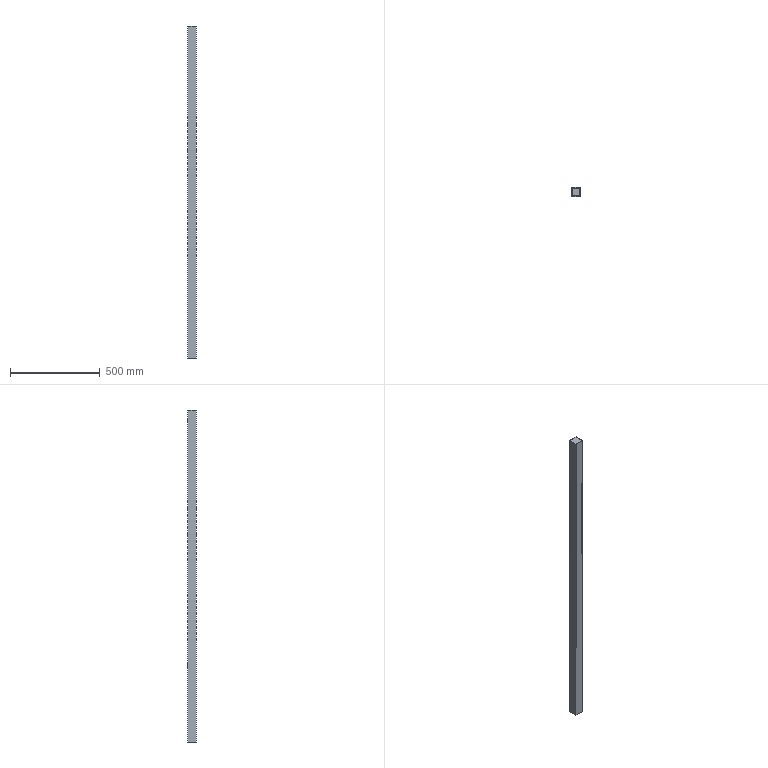Part | NX | features solid 2 | 1 solid | 15 faces | box 50 x 50 x 1848 mm | volume 1663845 mm3 | plane 11 | cylinder 4 | commonest cylinder face diameters 23 x4
STEP:
#1=CARTESIAN_POINT('',(585.,45.,1242.));
#2=VERTEX_POINT('',#1);
#3=CARTESIAN_POINT('',(625.,45.,1242.));
#4=VERTEX_POINT('',#3);
#5=CARTESIAN_POINT('',(585.,45.,1242.));
#6=DIRECTION('',(1.,0.,0.));
#7=VECTOR('',#6,1000.);
#8=LINE('',#5,#7);
#9=EDGE_CURVE('',#2,#4,#8,.T.);
#10=ORIENTED_EDGE('',*,*,#9,.T.);
#11=CARTESIAN_POINT('',(625.,5.,1242.));
#12=VERTEX_POINT('',#11);
#13=CARTESIAN_POINT('',(625.,45.,1242.));
#14=DIRECTION('',(0.,-1.,0.));
#15=VECTOR('',#14,1000.);
#16=LINE('',#13,#15);
#17=EDGE_CURVE('',#4,#12,#16,.T.);
#18=ORIENTED_EDGE('',*,*,#17,.T.);
#19=CARTESIAN_POINT('',(585.,5.,1242.));
#20=VERTEX_POINT('',#19);
#21=CARTESIAN_POINT('',(625.,5.,1242.));
#22=DIRECTION('',(-1.,0.,0.));
#23=VECTOR('',#22,1000.);
#24=LINE('',#21,#23);
#25=EDGE_CURVE('',#12,#20,#24,.T.);
#26=ORIENTED_EDGE('',*,*,#25,.T.);
#27=CARTESIAN_POINT('',(585.,5.,1242.));
#28=DIRECTION('',(0.,1.,0.));
#29=VECTOR('',#28,1000.);
#30=LINE('',#27,#29);
#31=EDGE_CURVE('',#20,#2,#30,.T.);
#32=ORIENTED_EDGE('',*,*,#31,.T.);
#33=EDGE_LOOP('',(#10,#18,#26,#32));
#34=FACE_BOUND('',#33,.T.);
#35=CARTESIAN_POINT('',(599.602,52.326,1242.));
#36=DIRECTION('',(0.,0.,-1.));
#37=DIRECTION('',(-1.,0.,0.));
#38=AXIS2_PLACEMENT_3D('',#35,#36,#37);
#39=PLANE('',#38);
#40=ADVANCED_FACE('',(#34),#39,.T.);
#41=CARTESIAN_POINT('',(605.,45.,1199.5));
#42=VERTEX_POINT('',#41);
#43=CARTESIAN_POINT('',(605.,50.,1199.5));
#44=VERTEX_POINT('',#43);
#45=CARTESIAN_POINT('',(605.,-1799.352,1199.5));
#46=DIRECTION('',(0.,1.,0.));
#47=VECTOR('',#46,1000.);
#48=LINE('',#45,#47);
#49=EDGE_CURVE('',#42,#44,#48,.T.);
#50=ORIENTED_EDGE('',*,*,#49,.F.);
#51=CARTESIAN_POINT('',(605.,45.,1176.5));
#52=VERTEX_POINT('',#51);
#53=CARTESIAN_POINT('',(605.,45.,1188.));
#54=DIRECTION('',(0.,-1.,0.));
#55=DIRECTION('',(0.,0.,1.));
#56=AXIS2_PLACEMENT_3D('',#53,#54,#55);
#57=CIRCLE('',#56,11.5);
#58=EDGE_CURVE('',#42,#52,#57,.T.);
#59=ORIENTED_EDGE('',*,*,#58,.T.);
#60=CARTESIAN_POINT('',(605.,50.,1176.5));
#61=VERTEX_POINT('',#60);
#62=CARTESIAN_POINT('',(605.,-1799.352,1176.5));
#63=DIRECTION('',(0.,1.,0.));
#64=VECTOR('',#63,1000.);
#65=LINE('',#62,#64);
#66=EDGE_CURVE('',#61,#52,#65,.F.);
#67=ORIENTED_EDGE('',*,*,#66,.F.);
#68=CARTESIAN_POINT('',(605.,50.,1188.));
#69=DIRECTION('',(0.,1.,0.));
#70=DIRECTION('',(0.,0.,1.));
#71=AXIS2_PLACEMENT_3D('',#68,#69,#70);
#72=CIRCLE('',#71,11.5);
#73=EDGE_CURVE('',#61,#44,#72,.T.);
#74=ORIENTED_EDGE('',*,*,#73,.T.);
#75=EDGE_LOOP('',(#50,#59,#67,#74));
#76=FACE_BOUND('',#75,.T.);
#77=CARTESIAN_POINT('',(605.,-1799.352,1188.));
#78=DIRECTION('',(0.,1.,0.));
#79=DIRECTION('',(0.,0.,-1.));
#80=AXIS2_PLACEMENT_3D('',#77,#78,#79);
#81=CYLINDRICAL_SURFACE('',#80,11.5);
#82=ADVANCED_FACE('',(#76),#81,.F.);
#83=CARTESIAN_POINT('',(605.,50.,-168.5));
#84=VERTEX_POINT('',#83);
#85=CARTESIAN_POINT('',(605.,45.,-168.5));
#86=VERTEX_POINT('',#85);
#87=CARTESIAN_POINT('',(605.,-1799.352,-168.5));
#88=DIRECTION('',(0.,1.,0.));
#89=VECTOR('',#88,1000.);
#90=LINE('',#87,#89);
#91=EDGE_CURVE('',#84,#86,#90,.F.);
#92=ORIENTED_EDGE('',*,*,#91,.T.);
#93=CARTESIAN_POINT('',(605.,45.,-191.5));
#94=VERTEX_POINT('',#93);
#95=CARTESIAN_POINT('',(605.,45.,-180.));
#96=DIRECTION('',(0.,-1.,0.));
#97=DIRECTION('',(0.,0.,1.));
#98=AXIS2_PLACEMENT_3D('',#95,#96,#97);
#99=CIRCLE('',#98,11.5);
#100=EDGE_CURVE('',#86,#94,#99,.T.);
#101=ORIENTED_EDGE('',*,*,#100,.T.);
#102=CARTESIAN_POINT('',(605.,50.,-191.5));
#103=VERTEX_POINT('',#102);
#104=CARTESIAN_POINT('',(605.,-1799.352,-191.5));
#105=DIRECTION('',(0.,1.,0.));
#106=VECTOR('',#105,1000.);
#107=LINE('',#104,#106);
#108=EDGE_CURVE('',#94,#103,#107,.T.);
#109=ORIENTED_EDGE('',*,*,#108,.T.);
#110=CARTESIAN_POINT('',(605.,50.,-180.));
#111=DIRECTION('',(0.,1.,0.));
#112=DIRECTION('',(0.,0.,1.));
#113=AXIS2_PLACEMENT_3D('',#110,#111,#112);
#114=CIRCLE('',#113,11.5);
#115=EDGE_CURVE('',#103,#84,#114,.T.);
#116=ORIENTED_EDGE('',*,*,#115,.T.);
#117=EDGE_LOOP('',(#92,#101,#109,#116));
#118=FACE_BOUND('',#117,.T.);
#119=CARTESIAN_POINT('',(605.,-1799.352,-180.));
#120=DIRECTION('',(0.,1.,0.));
#121=DIRECTION('',(0.,0.,-1.));
#122=AXIS2_PLACEMENT_3D('',#119,#120,#121);
#123=CYLINDRICAL_SURFACE('',#122,11.5);
#124=ADVANCED_FACE('',(#118),#123,.F.);
#125=ORIENTED_EDGE('',*,*,#115,.F.);
#126=CARTESIAN_POINT('',(605.,50.,-180.));
#127=DIRECTION('',(0.,1.,0.));
#128=DIRECTION('',(0.,0.,1.));
#129=AXIS2_PLACEMENT_3D('',#126,#127,#128);
#130=CIRCLE('',#129,11.5);
#131=EDGE_CURVE('',#84,#103,#130,.T.);
#132=ORIENTED_EDGE('',*,*,#131,.F.);
#133=EDGE_LOOP('',(#125,#132));
#134=FACE_BOUND('',#133,.T.);
#135=ORIENTED_EDGE('',*,*,#73,.F.);
#136=CARTESIAN_POINT('',(605.,50.,1188.));
#137=DIRECTION('',(0.,1.,0.));
#138=DIRECTION('',(0.,0.,1.));
#139=AXIS2_PLACEMENT_3D('',#136,#137,#138);
#140=CIRCLE('',#139,11.5);
#141=EDGE_CURVE('',#44,#61,#140,.T.);
#142=ORIENTED_EDGE('',*,*,#141,.F.);
#143=EDGE_LOOP('',(#135,#142));
#144=FACE_BOUND('',#143,.T.);
#145=CARTESIAN_POINT('',(580.,50.,-603.));
#146=VERTEX_POINT('',#145);
#147=CARTESIAN_POINT('',(580.,50.,1245.));
#148=VERTEX_POINT('',#147);
#149=CARTESIAN_POINT('',(580.,50.,-495.));
#150=DIRECTION('',(0.,0.,1.));
#151=VECTOR('',#150,1000.);
#152=LINE('',#149,#151);
#153=EDGE_CURVE('',#146,#148,#152,.T.);
#154=ORIENTED_EDGE('',*,*,#153,.T.);
#155=CARTESIAN_POINT('',(630.,50.,1245.));
#156=VERTEX_POINT('',#155);
#157=CARTESIAN_POINT('',(580.,50.,1245.));
#158=DIRECTION('',(-1.,0.,0.));
#159=VECTOR('',#158,1000.);
#160=LINE('',#157,#159);
#161=EDGE_CURVE('',#156,#148,#160,.T.);
#162=ORIENTED_EDGE('',*,*,#161,.F.);
#163=CARTESIAN_POINT('',(630.,50.,-603.));
#164=VERTEX_POINT('',#163);
#165=CARTESIAN_POINT('',(630.,50.,-495.));
#166=DIRECTION('',(0.,0.,-1.));
#167=VECTOR('',#166,1000.);
#168=LINE('',#165,#167);
#169=EDGE_CURVE('',#156,#164,#168,.T.);
#170=ORIENTED_EDGE('',*,*,#169,.T.);
#171=CARTESIAN_POINT('',(580.,50.,-603.));
#172=DIRECTION('',(-1.,0.,0.));
#173=VECTOR('',#172,1000.);
#174=LINE('',#171,#173);
#175=EDGE_CURVE('',#164,#146,#174,.T.);
#176=ORIENTED_EDGE('',*,*,#175,.T.);
#177=EDGE_LOOP('',(#154,#162,#170,#176));
#178=FACE_BOUND('',#177,.T.);
#179=CARTESIAN_POINT('',(580.,50.,-495.));
#180=DIRECTION('',(0.,-1.,0.));
#181=DIRECTION('',(-1.,0.,0.));
#182=AXIS2_PLACEMENT_3D('',#179,#180,#181);
#183=PLANE('',#182);
#184=ADVANCED_FACE('',(#134,#144,#178),#183,.F.);
#185=CARTESIAN_POINT('',(605.,45.,-180.));
#186=DIRECTION('',(0.,-1.,0.));
#187=DIRECTION('',(0.,0.,1.));
#188=AXIS2_PLACEMENT_3D('',#185,#186,#187);
#189=CIRCLE('',#188,11.5);
#190=EDGE_CURVE('',#94,#86,#189,.T.);
#191=ORIENTED_EDGE('',*,*,#190,.F.);
#192=ORIENTED_EDGE('',*,*,#100,.F.);
#193=EDGE_LOOP('',(#191,#192));
#194=FACE_BOUND('',#193,.T.);
#195=CARTESIAN_POINT('',(605.,45.,1188.));
#196=DIRECTION('',(0.,-1.,0.));
#197=DIRECTION('',(0.,0.,1.));
#198=AXIS2_PLACEMENT_3D('',#195,#196,#197);
#199=CIRCLE('',#198,11.5);
#200=EDGE_CURVE('',#52,#42,#199,.T.);
#201=ORIENTED_EDGE('',*,*,#200,.F.);
#202=ORIENTED_EDGE('',*,*,#58,.F.);
#203=EDGE_LOOP('',(#201,#202));
#204=FACE_BOUND('',#203,.T.);
#205=ORIENTED_EDGE('',*,*,#9,.F.);
#206=CARTESIAN_POINT('',(585.,45.,-603.));
#207=VERTEX_POINT('',#206);
#208=CARTESIAN_POINT('',(585.,45.,-495.));
#209=DIRECTION('',(0.,0.,1.));
#210=VECTOR('',#209,1000.);
#211=LINE('',#208,#210);
#212=EDGE_CURVE('',#207,#2,#211,.T.);
#213=ORIENTED_EDGE('',*,*,#212,.F.);
#214=CARTESIAN_POINT('',(625.,45.,-603.));
#215=VERTEX_POINT('',#214);
#216=CARTESIAN_POINT('',(630.,45.,-603.));
#217=DIRECTION('',(1.,0.,0.));
#218=VECTOR('',#217,1000.);
#219=LINE('',#216,#218);
#220=EDGE_CURVE('',#207,#215,#219,.T.);
#221=ORIENTED_EDGE('',*,*,#220,.T.);
#222=CARTESIAN_POINT('',(625.,45.,-495.));
#223=DIRECTION('',(0.,0.,-1.));
#224=VECTOR('',#223,1000.);
#225=LINE('',#222,#224);
#226=EDGE_CURVE('',#4,#215,#225,.T.);
#227=ORIENTED_EDGE('',*,*,#226,.F.);
#228=EDGE_LOOP('',(#205,#213,#221,#227));
#229=FACE_BOUND('',#228,.T.);
#230=CARTESIAN_POINT('',(585.,45.,-495.));
#231=DIRECTION('',(0.,-1.,0.));
#232=DIRECTION('',(-1.,0.,0.));
#233=AXIS2_PLACEMENT_3D('',#230,#231,#232);
#234=PLANE('',#233);
#235=ADVANCED_FACE('',(#194,#204,#229),#234,.T.);
#236=CARTESIAN_POINT('',(580.,0.,-603.));
#237=VERTEX_POINT('',#236);
#238=CARTESIAN_POINT('',(580.,0.,1245.));
#239=VERTEX_POINT('',#238);
#240=CARTESIAN_POINT('',(580.,0.,1245.));
#241=DIRECTION('',(0.,0.,1.));
#242=VECTOR('',#241,1000.);
#243=LINE('',#240,#242);
#244=EDGE_CURVE('',#237,#239,#243,.T.);
#245=ORIENTED_EDGE('',*,*,#244,.T.);
#246=CARTESIAN_POINT('',(580.,0.,1245.));
#247=DIRECTION('',(0.,-1.,0.));
#248=VECTOR('',#247,1000.);
#249=LINE('',#246,#248);
#250=EDGE_CURVE('',#148,#239,#249,.T.);
#251=ORIENTED_EDGE('',*,*,#250,.F.);
#252=ORIENTED_EDGE('',*,*,#153,.F.);
#253=CARTESIAN_POINT('',(580.,0.,-603.));
#254=DIRECTION('',(0.,-1.,0.));
#255=VECTOR('',#254,1000.);
#256=LINE('',#253,#255);
#257=EDGE_CURVE('',#146,#237,#256,.T.);
#258=ORIENTED_EDGE('',*,*,#257,.T.);
#259=EDGE_LOOP('',(#245,#251,#252,#258));
#260=FACE_BOUND('',#259,.T.);
#261=CARTESIAN_POINT('',(580.,0.,1245.));
#262=DIRECTION('',(1.,0.,0.));
#263=DIRECTION('',(0.,-1.,0.));
#264=AXIS2_PLACEMENT_3D('',#261,#262,#263);
#265=PLANE('',#264);
#266=ADVANCED_FACE('',(#260),#265,.F.);
#267=ORIENTED_EDGE('',*,*,#169,.F.);
#268=CARTESIAN_POINT('',(630.,0.,1245.));
#269=VERTEX_POINT('',#268);
#270=CARTESIAN_POINT('',(630.,0.,1245.));
#271=DIRECTION('',(0.,1.,0.));
#272=VECTOR('',#271,1000.);
#273=LINE('',#270,#272);
#274=EDGE_CURVE('',#269,#156,#273,.T.);
#275=ORIENTED_EDGE('',*,*,#274,.F.);
#276=CARTESIAN_POINT('',(630.,0.,-603.));
#277=VERTEX_POINT('',#276);
#278=CARTESIAN_POINT('',(630.,0.,-495.));
#279=DIRECTION('',(0.,0.,-1.));
#280=VECTOR('',#279,1000.);
#281=LINE('',#278,#280);
#282=EDGE_CURVE('',#269,#277,#281,.T.);
#283=ORIENTED_EDGE('',*,*,#282,.T.);
#284=CARTESIAN_POINT('',(630.,0.,-603.));
#285=DIRECTION('',(0.,1.,0.));
#286=VECTOR('',#285,1000.);
#287=LINE('',#284,#286);
#288=EDGE_CURVE('',#277,#164,#287,.T.);
#289=ORIENTED_EDGE('',*,*,#288,.T.);
#290=EDGE_LOOP('',(#267,#275,#283,#289));
#291=FACE_BOUND('',#290,.T.);
#292=CARTESIAN_POINT('',(630.,0.,-495.));
#293=DIRECTION('',(-1.,0.,0.));
#294=DIRECTION('',(0.,0.,1.));
#295=AXIS2_PLACEMENT_3D('',#292,#293,#294);
#296=PLANE('',#295);
#297=ADVANCED_FACE('',(#291),#296,.F.);
#298=CARTESIAN_POINT('',(625.,5.,-603.));
#299=VERTEX_POINT('',#298);
#300=CARTESIAN_POINT('',(625.,0.,-603.));
#301=DIRECTION('',(0.,-1.,0.));
#302=VECTOR('',#301,1000.);
#303=LINE('',#300,#302);
#304=EDGE_CURVE('',#215,#299,#303,.T.);
#305=ORIENTED_EDGE('',*,*,#304,.F.);
#306=ORIENTED_EDGE('',*,*,#220,.F.);
#307=CARTESIAN_POINT('',(585.,5.,-603.));
#308=VERTEX_POINT('',#307);
#309=CARTESIAN_POINT('',(585.,0.,-603.));
#310=DIRECTION('',(0.,1.,0.));
#311=VECTOR('',#310,1000.);
#312=LINE('',#309,#311);
#313=EDGE_CURVE('',#308,#207,#312,.T.);
#314=ORIENTED_EDGE('',*,*,#313,.F.);
#315=CARTESIAN_POINT('',(630.,5.,-603.));
#316=DIRECTION('',(-1.,0.,0.));
#317=VECTOR('',#316,1000.);
#318=LINE('',#315,#317);
#319=EDGE_CURVE('',#299,#308,#318,.T.);
#320=ORIENTED_EDGE('',*,*,#319,.F.);
#321=EDGE_LOOP('',(#305,#306,#314,#320));
#322=FACE_BOUND('',#321,.T.);
#323=ORIENTED_EDGE('',*,*,#257,.F.);
#324=ORIENTED_EDGE('',*,*,#175,.F.);
#325=ORIENTED_EDGE('',*,*,#288,.F.);
#326=CARTESIAN_POINT('',(630.,0.,-603.));
#327=DIRECTION('',(-1.,0.,0.));
#328=VECTOR('',#327,1000.);
#329=LINE('',#326,#328);
#330=EDGE_CURVE('',#277,#237,#329,.T.);
#331=ORIENTED_EDGE('',*,*,#330,.T.);
#332=EDGE_LOOP('',(#323,#324,#325,#331));
#333=FACE_BOUND('',#332,.T.);
#334=CARTESIAN_POINT('',(630.,0.,-603.));
#335=DIRECTION('',(0.,0.,1.));
#336=DIRECTION('',(0.,-1.,0.));
#337=AXIS2_PLACEMENT_3D('',#334,#335,#336);
#338=PLANE('',#337);
#339=ADVANCED_FACE('',(#322,#333),#338,.F.);
#340=ORIENTED_EDGE('',*,*,#31,.F.);
#341=CARTESIAN_POINT('',(585.,5.,1245.));
#342=DIRECTION('',(0.,0.,1.));
#343=VECTOR('',#342,1000.);
#344=LINE('',#341,#343);
#345=EDGE_CURVE('',#308,#20,#344,.T.);
#346=ORIENTED_EDGE('',*,*,#345,.F.);
#347=ORIENTED_EDGE('',*,*,#313,.T.);
#348=ORIENTED_EDGE('',*,*,#212,.T.);
#349=EDGE_LOOP('',(#340,#346,#347,#348));
#350=FACE_BOUND('',#349,.T.);
#351=CARTESIAN_POINT('',(585.,5.,1245.));
#352=DIRECTION('',(1.,0.,0.));
#353=DIRECTION('',(0.,-1.,0.));
#354=AXIS2_PLACEMENT_3D('',#351,#352,#353);
#355=PLANE('',#354);
#356=ADVANCED_FACE('',(#350),#355,.T.);
#357=ORIENTED_EDGE('',*,*,#161,.T.);
#358=ORIENTED_EDGE('',*,*,#250,.T.);
#359=CARTESIAN_POINT('',(630.,0.,1245.));
#360=DIRECTION('',(1.,0.,0.));
#361=VECTOR('',#360,1000.);
#362=LINE('',#359,#361);
#363=EDGE_CURVE('',#239,#269,#362,.T.);
#364=ORIENTED_EDGE('',*,*,#363,.T.);
#365=ORIENTED_EDGE('',*,*,#274,.T.);
#366=EDGE_LOOP('',(#357,#358,#364,#365));
#367=FACE_BOUND('',#366,.T.);
#368=CARTESIAN_POINT('',(630.,0.,1245.));
#369=DIRECTION('',(0.,0.,1.));
#370=DIRECTION('',(0.,-1.,0.));
#371=AXIS2_PLACEMENT_3D('',#368,#369,#370);
#372=PLANE('',#371);
#373=ADVANCED_FACE('',(#367),#372,.T.);
#374=ORIENTED_EDGE('',*,*,#17,.F.);
#375=ORIENTED_EDGE('',*,*,#226,.T.);
#376=ORIENTED_EDGE('',*,*,#304,.T.);
#377=CARTESIAN_POINT('',(625.,5.,-495.));
#378=DIRECTION('',(0.,0.,-1.));
#379=VECTOR('',#378,1000.);
#380=LINE('',#377,#379);
#381=EDGE_CURVE('',#12,#299,#380,.T.);
#382=ORIENTED_EDGE('',*,*,#381,.F.);
#383=EDGE_LOOP('',(#374,#375,#376,#382));
#384=FACE_BOUND('',#383,.T.);
#385=CARTESIAN_POINT('',(625.,45.,-495.));
#386=DIRECTION('',(-1.,0.,0.));
#387=DIRECTION('',(0.,0.,1.));
#388=AXIS2_PLACEMENT_3D('',#385,#386,#387);
#389=PLANE('',#388);
#390=ADVANCED_FACE('',(#384),#389,.T.);
#391=ORIENTED_EDGE('',*,*,#282,.F.);
#392=ORIENTED_EDGE('',*,*,#363,.F.);
#393=ORIENTED_EDGE('',*,*,#244,.F.);
#394=ORIENTED_EDGE('',*,*,#330,.F.);
#395=EDGE_LOOP('',(#391,#392,#393,#394));
#396=FACE_BOUND('',#395,.T.);
#397=CARTESIAN_POINT('',(630.,0.,-495.));
#398=DIRECTION('',(0.,1.,0.));
#399=DIRECTION('',(1.,0.,0.));
#400=AXIS2_PLACEMENT_3D('',#397,#398,#399);
#401=PLANE('',#400);
#402=ADVANCED_FACE('',(#396),#401,.F.);
#403=ORIENTED_EDGE('',*,*,#25,.F.);
#404=ORIENTED_EDGE('',*,*,#381,.T.);
#405=ORIENTED_EDGE('',*,*,#319,.T.);
#406=ORIENTED_EDGE('',*,*,#345,.T.);
#407=EDGE_LOOP('',(#403,#404,#405,#406));
#408=FACE_BOUND('',#407,.T.);
#409=CARTESIAN_POINT('',(625.,5.,1245.));
#410=DIRECTION('',(0.,1.,0.));
#411=DIRECTION('',(1.,0.,0.));
#412=AXIS2_PLACEMENT_3D('',#409,#410,#411);
#413=PLANE('',#412);
#414=ADVANCED_FACE('',(#408),#413,.T.);
#415=ORIENTED_EDGE('',*,*,#190,.T.);
#416=ORIENTED_EDGE('',*,*,#91,.F.);
#417=ORIENTED_EDGE('',*,*,#131,.T.);
#418=ORIENTED_EDGE('',*,*,#108,.F.);
#419=EDGE_LOOP('',(#415,#416,#417,#418));
#420=FACE_BOUND('',#419,.T.);
#421=CARTESIAN_POINT('',(605.,-1799.352,-180.));
#422=DIRECTION('',(0.,1.,0.));
#423=DIRECTION('',(0.,0.,-1.));
#424=AXIS2_PLACEMENT_3D('',#421,#422,#423);
#425=CYLINDRICAL_SURFACE('',#424,11.5);
#426=ADVANCED_FACE('',(#420),#425,.F.);
#427=ORIENTED_EDGE('',*,*,#200,.T.);
#428=ORIENTED_EDGE('',*,*,#49,.T.);
#429=ORIENTED_EDGE('',*,*,#141,.T.);
#430=ORIENTED_EDGE('',*,*,#66,.T.);
#431=EDGE_LOOP('',(#427,#428,#429,#430));
#432=FACE_BOUND('',#431,.T.);
#433=CARTESIAN_POINT('',(605.,-1799.352,1188.));
#434=DIRECTION('',(0.,1.,0.));
#435=DIRECTION('',(0.,0.,-1.));
#436=AXIS2_PLACEMENT_3D('',#433,#434,#435);
#437=CYLINDRICAL_SURFACE('',#436,11.5);
#438=ADVANCED_FACE('',(#432),#437,.F.);
#439=CLOSED_SHELL('',(#40,#82,#124,#184,#235,#266,#297,#339,#356,#373,#390,#402,#414,#426,#438));
#440=MANIFOLD_SOLID_BREP('',#439);
#441=(LENGTH_UNIT()NAMED_UNIT(*)SI_UNIT(.MILLI.,.METRE.));
#442=UNCERTAINTY_MEASURE_WITH_UNIT(LENGTH_MEASURE(0.00001),#441,'','');
#443=(NAMED_UNIT(*)PLANE_ANGLE_UNIT()SI_UNIT($,.RADIAN.));
#444=(NAMED_UNIT(*)SI_UNIT($,.STERADIAN.)SOLID_ANGLE_UNIT());
#445=(GEOMETRIC_REPRESENTATION_CONTEXT(3)GLOBAL_UNCERTAINTY_ASSIGNED_CONTEXT((#442))GLOBAL_UNIT_ASSIGNED_CONTEXT((#441,#443,#444))REPRESENTATION_CONTEXT('',''));
#446=ADVANCED_BREP_SHAPE_REPRESENTATION('',(#440),#445);